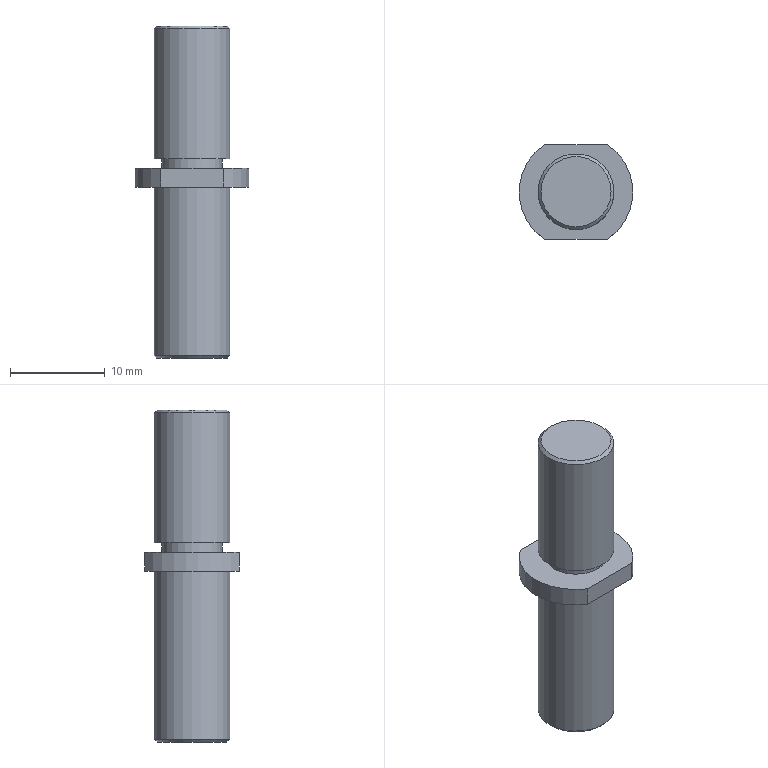Part | NX | 1 solid | 16 faces | box 12 x 10 x 35 mm | volume 1669 mm3 | plane 7 | cylinder 6 | cone 3 | commonest cylinder face diameters 8 x2 12 x2 4.2 x1 6.4 x1
STEP:
#1=CARTESIAN_POINT('',(3.317,-5.,2.));
#2=VERTEX_POINT('',#1);
#3=CARTESIAN_POINT('',(3.317,5.,2.));
#4=VERTEX_POINT('',#3);
#5=CARTESIAN_POINT('',(0.,0.,2.));
#6=DIRECTION('',(0.,0.,1.));
#7=DIRECTION('',(1.,0.,0.));
#8=AXIS2_PLACEMENT_3D('',#5,#6,#7);
#9=CIRCLE('',#8,6.);
#10=EDGE_CURVE('',#2,#4,#9,.T.);
#11=ORIENTED_EDGE('',*,*,#10,.F.);
#12=CARTESIAN_POINT('',(3.317,-5.,0.));
#13=VERTEX_POINT('',#12);
#14=CARTESIAN_POINT('',(3.317,-5.,2.));
#15=DIRECTION('',(0.,0.,-1.));
#16=VECTOR('',#15,1000.);
#17=LINE('',#14,#16);
#18=EDGE_CURVE('',#2,#13,#17,.T.);
#19=ORIENTED_EDGE('',*,*,#18,.T.);
#20=CARTESIAN_POINT('',(3.317,5.,0.));
#21=VERTEX_POINT('',#20);
#22=CARTESIAN_POINT('',(0.,0.,0.));
#23=DIRECTION('',(0.,0.,1.));
#24=DIRECTION('',(1.,0.,0.));
#25=AXIS2_PLACEMENT_3D('',#22,#23,#24);
#26=CIRCLE('',#25,6.);
#27=EDGE_CURVE('',#13,#21,#26,.T.);
#28=ORIENTED_EDGE('',*,*,#27,.T.);
#29=CARTESIAN_POINT('',(3.317,5.,2.));
#30=DIRECTION('',(0.,0.,-1.));
#31=VECTOR('',#30,1000.);
#32=LINE('',#29,#31);
#33=EDGE_CURVE('',#21,#4,#32,.F.);
#34=ORIENTED_EDGE('',*,*,#33,.T.);
#35=EDGE_LOOP('',(#11,#19,#28,#34));
#36=FACE_BOUND('',#35,.T.);
#37=CARTESIAN_POINT('',(0.,0.,2.));
#38=DIRECTION('',(0.,0.,-1.));
#39=DIRECTION('',(-1.,0.,0.));
#40=AXIS2_PLACEMENT_3D('',#37,#38,#39);
#41=CYLINDRICAL_SURFACE('',#40,6.);
#42=ADVANCED_FACE('',(#36),#41,.T.);
#43=CARTESIAN_POINT('',(-3.317,5.,0.));
#44=VERTEX_POINT('',#43);
#45=CARTESIAN_POINT('',(-3.317,-5.,0.));
#46=VERTEX_POINT('',#45);
#47=CARTESIAN_POINT('',(0.,0.,0.));
#48=DIRECTION('',(0.,0.,1.));
#49=DIRECTION('',(1.,0.,0.));
#50=AXIS2_PLACEMENT_3D('',#47,#48,#49);
#51=CIRCLE('',#50,6.);
#52=EDGE_CURVE('',#44,#46,#51,.T.);
#53=ORIENTED_EDGE('',*,*,#52,.T.);
#54=CARTESIAN_POINT('',(-3.317,-5.,2.));
#55=VERTEX_POINT('',#54);
#56=CARTESIAN_POINT('',(-3.317,-5.,2.));
#57=DIRECTION('',(0.,0.,-1.));
#58=VECTOR('',#57,1000.);
#59=LINE('',#56,#58);
#60=EDGE_CURVE('',#46,#55,#59,.F.);
#61=ORIENTED_EDGE('',*,*,#60,.T.);
#62=CARTESIAN_POINT('',(-3.317,5.,2.));
#63=VERTEX_POINT('',#62);
#64=CARTESIAN_POINT('',(0.,0.,2.));
#65=DIRECTION('',(0.,0.,1.));
#66=DIRECTION('',(1.,0.,0.));
#67=AXIS2_PLACEMENT_3D('',#64,#65,#66);
#68=CIRCLE('',#67,6.);
#69=EDGE_CURVE('',#63,#55,#68,.T.);
#70=ORIENTED_EDGE('',*,*,#69,.F.);
#71=CARTESIAN_POINT('',(-3.317,5.,2.));
#72=DIRECTION('',(0.,0.,-1.));
#73=VECTOR('',#72,1000.);
#74=LINE('',#71,#73);
#75=EDGE_CURVE('',#63,#44,#74,.T.);
#76=ORIENTED_EDGE('',*,*,#75,.T.);
#77=EDGE_LOOP('',(#53,#61,#70,#76));
#78=FACE_BOUND('',#77,.T.);
#79=CARTESIAN_POINT('',(0.,0.,2.));
#80=DIRECTION('',(0.,0.,-1.));
#81=DIRECTION('',(-1.,0.,0.));
#82=AXIS2_PLACEMENT_3D('',#79,#80,#81);
#83=CYLINDRICAL_SURFACE('',#82,6.);
#84=ADVANCED_FACE('',(#78),#83,.T.);
#85=CARTESIAN_POINT('',(0.,-5.,2.));
#86=DIRECTION('',(-1.,0.,0.));
#87=VECTOR('',#86,1000.);
#88=LINE('',#85,#87);
#89=EDGE_CURVE('',#2,#55,#88,.T.);
#90=ORIENTED_EDGE('',*,*,#89,.F.);
#91=ORIENTED_EDGE('',*,*,#10,.T.);
#92=CARTESIAN_POINT('',(0.,5.,2.));
#93=DIRECTION('',(1.,0.,0.));
#94=VECTOR('',#93,1000.);
#95=LINE('',#92,#94);
#96=EDGE_CURVE('',#63,#4,#95,.T.);
#97=ORIENTED_EDGE('',*,*,#96,.F.);
#98=ORIENTED_EDGE('',*,*,#69,.T.);
#99=EDGE_LOOP('',(#90,#91,#97,#98));
#100=FACE_BOUND('',#99,.T.);
#101=CARTESIAN_POINT('',(3.2,0.,2.));
#102=VERTEX_POINT('',#101);
#103=CARTESIAN_POINT('',(0.,0.,2.));
#104=DIRECTION('',(0.,0.,1.));
#105=DIRECTION('',(1.,0.,0.));
#106=AXIS2_PLACEMENT_3D('',#103,#104,#105);
#107=CIRCLE('',#106,3.2);
#108=EDGE_CURVE('',#102,#102,#107,.T.);
#109=ORIENTED_EDGE('',*,*,#108,.F.);
#110=EDGE_LOOP('',(#109));
#111=FACE_BOUND('',#110,.T.);
#112=CARTESIAN_POINT('',(0.,0.,2.));
#113=DIRECTION('',(0.,0.,1.));
#114=DIRECTION('',(1.,0.,0.));
#115=AXIS2_PLACEMENT_3D('',#112,#113,#114);
#116=PLANE('',#115);
#117=ADVANCED_FACE('',(#100,#111),#116,.T.);
#118=CARTESIAN_POINT('',(4.,0.,0.));
#119=VERTEX_POINT('',#118);
#120=CARTESIAN_POINT('',(0.,0.,0.));
#121=DIRECTION('',(0.,0.,1.));
#122=DIRECTION('',(1.,0.,0.));
#123=AXIS2_PLACEMENT_3D('',#120,#121,#122);
#124=CIRCLE('',#123,4.);
#125=EDGE_CURVE('',#119,#119,#124,.F.);
#126=ORIENTED_EDGE('',*,*,#125,.F.);
#127=EDGE_LOOP('',(#126));
#128=FACE_BOUND('',#127,.T.);
#129=ORIENTED_EDGE('',*,*,#27,.F.);
#130=CARTESIAN_POINT('',(0.,-5.,0.));
#131=DIRECTION('',(-1.,0.,0.));
#132=VECTOR('',#131,1000.);
#133=LINE('',#130,#132);
#134=EDGE_CURVE('',#13,#46,#133,.T.);
#135=ORIENTED_EDGE('',*,*,#134,.T.);
#136=ORIENTED_EDGE('',*,*,#52,.F.);
#137=CARTESIAN_POINT('',(0.,5.,0.));
#138=DIRECTION('',(1.,0.,0.));
#139=VECTOR('',#138,1000.);
#140=LINE('',#137,#139);
#141=EDGE_CURVE('',#44,#21,#140,.T.);
#142=ORIENTED_EDGE('',*,*,#141,.T.);
#143=EDGE_LOOP('',(#129,#135,#136,#142));
#144=FACE_BOUND('',#143,.T.);
#145=CARTESIAN_POINT('',(0.,0.,0.));
#146=DIRECTION('',(0.,0.,1.));
#147=DIRECTION('',(1.,0.,0.));
#148=AXIS2_PLACEMENT_3D('',#145,#146,#147);
#149=PLANE('',#148);
#150=ADVANCED_FACE('',(#128,#144),#149,.F.);
#151=CARTESIAN_POINT('',(3.7,0.,-18.));
#152=VERTEX_POINT('',#151);
#153=CARTESIAN_POINT('',(0.,0.,-18.));
#154=DIRECTION('',(0.,0.,1.));
#155=DIRECTION('',(1.,0.,0.));
#156=AXIS2_PLACEMENT_3D('',#153,#154,#155);
#157=CIRCLE('',#156,3.7);
#158=EDGE_CURVE('',#152,#152,#157,.F.);
#159=ORIENTED_EDGE('',*,*,#158,.T.);
#160=EDGE_LOOP('',(#159));
#161=FACE_BOUND('',#160,.T.);
#162=CARTESIAN_POINT('',(-2.1,0.,-18.));
#163=VERTEX_POINT('',#162);
#164=CARTESIAN_POINT('',(0.,0.,-18.));
#165=DIRECTION('',(0.,0.,-1.));
#166=DIRECTION('',(-1.,0.,0.));
#167=AXIS2_PLACEMENT_3D('',#164,#165,#166);
#168=CIRCLE('',#167,2.1);
#169=EDGE_CURVE('',#163,#163,#168,.T.);
#170=ORIENTED_EDGE('',*,*,#169,.F.);
#171=EDGE_LOOP('',(#170));
#172=FACE_BOUND('',#171,.T.);
#173=CARTESIAN_POINT('',(0.,0.,-18.));
#174=DIRECTION('',(0.,0.,1.));
#175=DIRECTION('',(1.,0.,0.));
#176=AXIS2_PLACEMENT_3D('',#173,#174,#175);
#177=PLANE('',#176);
#178=ADVANCED_FACE('',(#161,#172),#177,.F.);
#179=CARTESIAN_POINT('',(4.,0.,-17.7));
#180=VERTEX_POINT('',#179);
#181=CARTESIAN_POINT('',(0.,0.,-17.7));
#182=DIRECTION('',(0.,0.,1.));
#183=DIRECTION('',(1.,0.,0.));
#184=AXIS2_PLACEMENT_3D('',#181,#182,#183);
#185=CIRCLE('',#184,4.);
#186=EDGE_CURVE('',#180,#180,#185,.T.);
#187=ORIENTED_EDGE('',*,*,#186,.T.);
#188=EDGE_LOOP('',(#187));
#189=FACE_BOUND('',#188,.T.);
#190=ORIENTED_EDGE('',*,*,#125,.T.);
#191=EDGE_LOOP('',(#190));
#192=FACE_BOUND('',#191,.T.);
#193=CARTESIAN_POINT('',(0.,0.,-18.));
#194=DIRECTION('',(0.,0.,1.));
#195=DIRECTION('',(1.,0.,0.));
#196=AXIS2_PLACEMENT_3D('',#193,#194,#195);
#197=CYLINDRICAL_SURFACE('',#196,4.);
#198=ADVANCED_FACE('',(#189,#192),#197,.T.);
#199=CARTESIAN_POINT('',(4.,0.,3.));
#200=VERTEX_POINT('',#199);
#201=CARTESIAN_POINT('',(0.,0.,3.));
#202=DIRECTION('',(0.,0.,1.));
#203=DIRECTION('',(1.,0.,0.));
#204=AXIS2_PLACEMENT_3D('',#201,#202,#203);
#205=CIRCLE('',#204,4.);
#206=EDGE_CURVE('',#200,#200,#205,.T.);
#207=ORIENTED_EDGE('',*,*,#206,.F.);
#208=EDGE_LOOP('',(#207));
#209=FACE_BOUND('',#208,.T.);
#210=CARTESIAN_POINT('',(3.2,0.,3.));
#211=VERTEX_POINT('',#210);
#212=CARTESIAN_POINT('',(0.,0.,3.));
#213=DIRECTION('',(0.,0.,1.));
#214=DIRECTION('',(1.,0.,0.));
#215=AXIS2_PLACEMENT_3D('',#212,#213,#214);
#216=CIRCLE('',#215,3.2);
#217=EDGE_CURVE('',#211,#211,#216,.T.);
#218=ORIENTED_EDGE('',*,*,#217,.T.);
#219=EDGE_LOOP('',(#218));
#220=FACE_BOUND('',#219,.T.);
#221=CARTESIAN_POINT('',(4.,0.,3.));
#222=DIRECTION('',(0.,0.,1.));
#223=DIRECTION('',(1.,0.,0.));
#224=AXIS2_PLACEMENT_3D('',#221,#222,#223);
#225=PLANE('',#224);
#226=ADVANCED_FACE('',(#209,#220),#225,.F.);
#227=ORIENTED_EDGE('',*,*,#217,.F.);
#228=EDGE_LOOP('',(#227));
#229=FACE_BOUND('',#228,.T.);
#230=ORIENTED_EDGE('',*,*,#108,.T.);
#231=EDGE_LOOP('',(#230));
#232=FACE_BOUND('',#231,.T.);
#233=CARTESIAN_POINT('',(0.,0.,0.));
#234=DIRECTION('',(0.,0.,1.));
#235=DIRECTION('',(1.,0.,0.));
#236=AXIS2_PLACEMENT_3D('',#233,#234,#235);
#237=CYLINDRICAL_SURFACE('',#236,3.2);
#238=ADVANCED_FACE('',(#229,#232),#237,.T.);
#239=CARTESIAN_POINT('',(3.7,0.,17.));
#240=VERTEX_POINT('',#239);
#241=CARTESIAN_POINT('',(0.,0.,17.));
#242=DIRECTION('',(0.,0.,1.));
#243=DIRECTION('',(1.,0.,0.));
#244=AXIS2_PLACEMENT_3D('',#241,#242,#243);
#245=CIRCLE('',#244,3.7);
#246=EDGE_CURVE('',#240,#240,#245,.T.);
#247=ORIENTED_EDGE('',*,*,#246,.T.);
#248=EDGE_LOOP('',(#247));
#249=FACE_BOUND('',#248,.T.);
#250=CARTESIAN_POINT('',(0.,0.,17.));
#251=DIRECTION('',(0.,0.,1.));
#252=DIRECTION('',(1.,0.,0.));
#253=AXIS2_PLACEMENT_3D('',#250,#251,#252);
#254=PLANE('',#253);
#255=ADVANCED_FACE('',(#249),#254,.T.);
#256=CARTESIAN_POINT('',(4.,0.,16.7));
#257=VERTEX_POINT('',#256);
#258=CARTESIAN_POINT('',(0.,0.,16.7));
#259=DIRECTION('',(0.,0.,1.));
#260=DIRECTION('',(1.,0.,0.));
#261=AXIS2_PLACEMENT_3D('',#258,#259,#260);
#262=CIRCLE('',#261,4.);
#263=EDGE_CURVE('',#257,#257,#262,.F.);
#264=ORIENTED_EDGE('',*,*,#263,.T.);
#265=EDGE_LOOP('',(#264));
#266=FACE_BOUND('',#265,.T.);
#267=ORIENTED_EDGE('',*,*,#206,.T.);
#268=EDGE_LOOP('',(#267));
#269=FACE_BOUND('',#268,.T.);
#270=CARTESIAN_POINT('',(0.,0.,-18.));
#271=DIRECTION('',(0.,0.,1.));
#272=DIRECTION('',(1.,0.,0.));
#273=AXIS2_PLACEMENT_3D('',#270,#271,#272);
#274=CYLINDRICAL_SURFACE('',#273,4.);
#275=ADVANCED_FACE('',(#266,#269),#274,.T.);
#276=CARTESIAN_POINT('',(0.,0.,-4.338));
#277=VERTEX_POINT('',#276);
#278=VERTEX_LOOP('',#277);
#279=FACE_BOUND('',#278,.T.);
#280=CARTESIAN_POINT('',(-2.1,0.,-5.6));
#281=VERTEX_POINT('',#280);
#282=CARTESIAN_POINT('',(0.,0.,-5.6));
#283=DIRECTION('',(0.,0.,-1.));
#284=DIRECTION('',(-1.,0.,0.));
#285=AXIS2_PLACEMENT_3D('',#282,#283,#284);
#286=CIRCLE('',#285,2.1);
#287=EDGE_CURVE('',#281,#281,#286,.T.);
#288=ORIENTED_EDGE('',*,*,#287,.T.);
#289=EDGE_LOOP('',(#288));
#290=FACE_BOUND('',#289,.T.);
#291=CARTESIAN_POINT('',(0.,0.,-5.6));
#292=DIRECTION('',(0.,0.,-1.));
#293=DIRECTION('',(-1.,0.,0.));
#294=AXIS2_PLACEMENT_3D('',#291,#292,#293);
#295=CONICAL_SURFACE('',#294,2.1,1.03);
#296=ADVANCED_FACE('',(#279,#290),#295,.F.);
#297=ORIENTED_EDGE('',*,*,#287,.F.);
#298=EDGE_LOOP('',(#297));
#299=FACE_BOUND('',#298,.T.);
#300=ORIENTED_EDGE('',*,*,#169,.T.);
#301=EDGE_LOOP('',(#300));
#302=FACE_BOUND('',#301,.T.);
#303=CARTESIAN_POINT('',(0.,0.,-18.));
#304=DIRECTION('',(0.,0.,-1.));
#305=DIRECTION('',(-1.,0.,0.));
#306=AXIS2_PLACEMENT_3D('',#303,#304,#305);
#307=CYLINDRICAL_SURFACE('',#306,2.1);
#308=ADVANCED_FACE('',(#299,#302),#307,.F.);
#309=ORIENTED_EDGE('',*,*,#158,.F.);
#310=EDGE_LOOP('',(#309));
#311=FACE_BOUND('',#310,.T.);
#312=ORIENTED_EDGE('',*,*,#186,.F.);
#313=EDGE_LOOP('',(#312));
#314=FACE_BOUND('',#313,.T.);
#315=CARTESIAN_POINT('',(0.,0.,-17.7));
#316=DIRECTION('',(0.,0.,1.));
#317=DIRECTION('',(1.,0.,0.));
#318=AXIS2_PLACEMENT_3D('',#315,#316,#317);
#319=CONICAL_SURFACE('',#318,4.,0.7854);
#320=ADVANCED_FACE('',(#311,#314),#319,.T.);
#321=ORIENTED_EDGE('',*,*,#263,.F.);
#322=EDGE_LOOP('',(#321));
#323=FACE_BOUND('',#322,.T.);
#324=ORIENTED_EDGE('',*,*,#246,.F.);
#325=EDGE_LOOP('',(#324));
#326=FACE_BOUND('',#325,.T.);
#327=CARTESIAN_POINT('',(0.,0.,17.));
#328=DIRECTION('',(0.,0.,-1.));
#329=DIRECTION('',(-1.,0.,0.));
#330=AXIS2_PLACEMENT_3D('',#327,#328,#329);
#331=CONICAL_SURFACE('',#330,3.7,0.7854);
#332=ADVANCED_FACE('',(#323,#326),#331,.T.);
#333=ORIENTED_EDGE('',*,*,#96,.T.);
#334=ORIENTED_EDGE('',*,*,#33,.F.);
#335=ORIENTED_EDGE('',*,*,#141,.F.);
#336=ORIENTED_EDGE('',*,*,#75,.F.);
#337=EDGE_LOOP('',(#333,#334,#335,#336));
#338=FACE_BOUND('',#337,.T.);
#339=CARTESIAN_POINT('',(6.679,5.,17.));
#340=DIRECTION('',(0.,-1.,0.));
#341=DIRECTION('',(0.,0.,-1.));
#342=AXIS2_PLACEMENT_3D('',#339,#340,#341);
#343=PLANE('',#342);
#344=ADVANCED_FACE('',(#338),#343,.F.);
#345=ORIENTED_EDGE('',*,*,#89,.T.);
#346=ORIENTED_EDGE('',*,*,#60,.F.);
#347=ORIENTED_EDGE('',*,*,#134,.F.);
#348=ORIENTED_EDGE('',*,*,#18,.F.);
#349=EDGE_LOOP('',(#345,#346,#347,#348));
#350=FACE_BOUND('',#349,.T.);
#351=CARTESIAN_POINT('',(6.679,-5.,17.));
#352=DIRECTION('',(0.,1.,0.));
#353=DIRECTION('',(0.,0.,1.));
#354=AXIS2_PLACEMENT_3D('',#351,#352,#353);
#355=PLANE('',#354);
#356=ADVANCED_FACE('',(#350),#355,.F.);
#357=CLOSED_SHELL('',(#42,#84,#117,#150,#178,#198,#226,#238,#255,#275,#296,#308,#320,#332,#344,#356));
#358=MANIFOLD_SOLID_BREP('',#357);
#359=(LENGTH_UNIT()NAMED_UNIT(*)SI_UNIT(.MILLI.,.METRE.));
#360=UNCERTAINTY_MEASURE_WITH_UNIT(LENGTH_MEASURE(0.00001),#359,'','');
#361=(NAMED_UNIT(*)PLANE_ANGLE_UNIT()SI_UNIT($,.RADIAN.));
#362=(NAMED_UNIT(*)SI_UNIT($,.STERADIAN.)SOLID_ANGLE_UNIT());
#363=(GEOMETRIC_REPRESENTATION_CONTEXT(3)GLOBAL_UNCERTAINTY_ASSIGNED_CONTEXT((#360))GLOBAL_UNIT_ASSIGNED_CONTEXT((#359,#361,#362))REPRESENTATION_CONTEXT('',''));
#364=ADVANCED_BREP_SHAPE_REPRESENTATION('',(#358),#363);